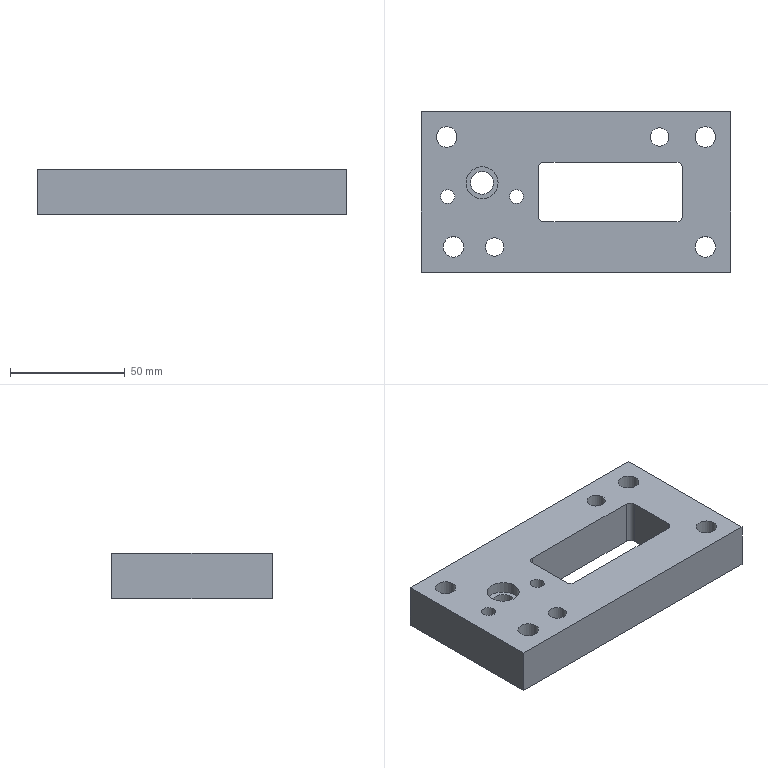Part | STEP file | 429_id2790_x_t | 1 solid | 42 faces | box 135 x 70 x 20 mm | volume 140686 mm3 | cylinder 20 | plane 17 | spline 5 | commonest cylinder face diameters 9 x6 14 x5 5 x4 6.1 x2 8 x2 10 x1